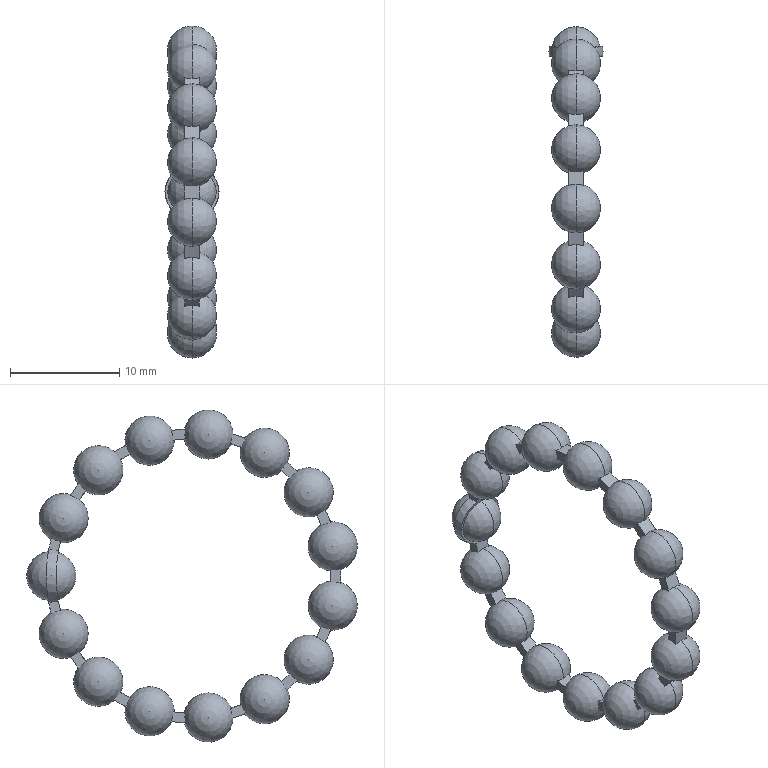Part | SolidWorks | features BaseBody 1 | 1 solid | 92 faces | box 4.95 x 30.216 x 30.358 mm | volume 737.087 mm3 | sphere 34 | plane 30 | cylinder 28 | commonest cylinder face diameters 25.1 x14 26.9 x14